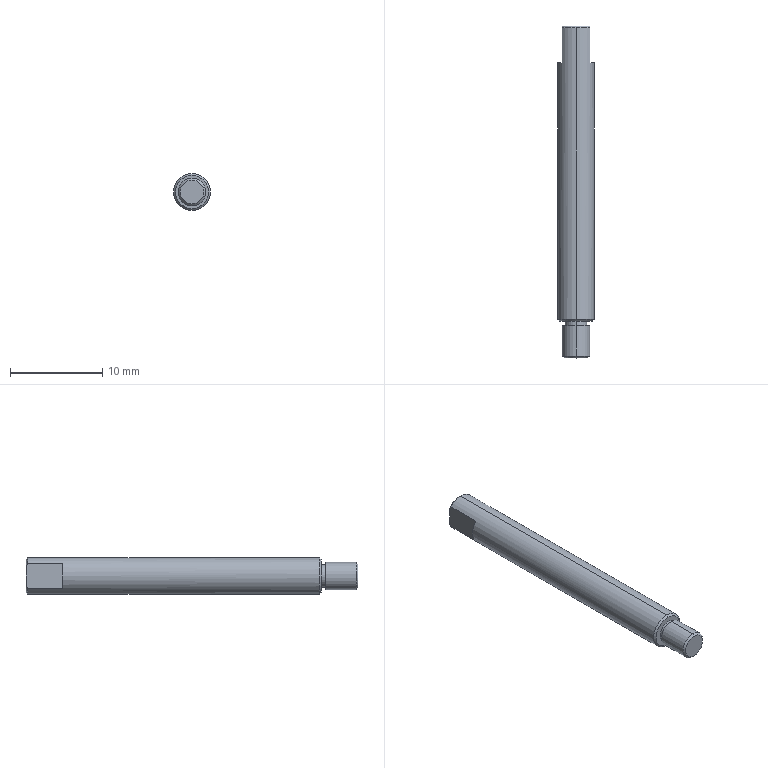Part | STEP file | 10000054026swp000-1 | 1 solid | 21 faces | box 4 x 36 x 4 mm | volume 421.312 mm3 | plane 8 | cone 7 | cylinder 6 | commonest cylinder face diameters 2.4 x2 3 x2 4 x2
STEP:
#1=CARTESIAN_POINT('',(0.,0.,-1.3));
#2=VERTEX_POINT('',#1);
#3=CARTESIAN_POINT('',(0.,0.,1.3));
#4=VERTEX_POINT('',#3);
#5=CARTESIAN_POINT('',(0.,0.,0.));
#6=DIRECTION('',(0.,-1.,0.));
#7=DIRECTION('',(0.,0.,1.));
#8=AXIS2_PLACEMENT_3D('',#5,#6,#7);
#9=CIRCLE('',#8,1.3);
#10=EDGE_CURVE('',#2,#4,#9,.T.);
#11=ORIENTED_EDGE('',*,*,#10,.F.);
#12=CARTESIAN_POINT('',(0.,0.2,-1.5));
#13=VERTEX_POINT('',#12);
#14=CARTESIAN_POINT('',(0.,0.2,-1.5));
#15=DIRECTION('',(0.,0.7071,-0.7071));
#16=VECTOR('',#15,1000.);
#17=LINE('',#14,#16);
#18=EDGE_CURVE('',#2,#13,#17,.T.);
#19=ORIENTED_EDGE('',*,*,#18,.T.);
#20=CARTESIAN_POINT('',(0.,0.2,1.5));
#21=VERTEX_POINT('',#20);
#22=CARTESIAN_POINT('',(0.,0.2,0.));
#23=DIRECTION('',(0.,1.,0.));
#24=DIRECTION('',(0.,0.,1.));
#25=AXIS2_PLACEMENT_3D('',#22,#23,#24);
#26=CIRCLE('',#25,1.5);
#27=EDGE_CURVE('',#21,#13,#26,.T.);
#28=ORIENTED_EDGE('',*,*,#27,.F.);
#29=CARTESIAN_POINT('',(0.,0.2,1.5));
#30=DIRECTION('',(0.,0.7071,0.7071));
#31=VECTOR('',#30,1000.);
#32=LINE('',#29,#31);
#33=EDGE_CURVE('',#4,#21,#32,.T.);
#34=ORIENTED_EDGE('',*,*,#33,.F.);
#35=EDGE_LOOP('',(#11,#19,#28,#34));
#36=FACE_OUTER_BOUND('',#35,.T.);
#37=CARTESIAN_POINT('',(0.,0.2,0.));
#38=DIRECTION('',(0.,1.,0.));
#39=DIRECTION('',(0.,0.,1.));
#40=AXIS2_PLACEMENT_3D('',#37,#38,#39);
#41=CONICAL_SURFACE('',#40,1.5,0.7854);
#42=ADVANCED_FACE('',(#36),#41,.T.);
#43=CARTESIAN_POINT('',(0.,4.,-1.8));
#44=VERTEX_POINT('',#43);
#45=CARTESIAN_POINT('',(0.,4.,1.8));
#46=VERTEX_POINT('',#45);
#47=CARTESIAN_POINT('',(0.,4.,0.));
#48=DIRECTION('',(0.,-1.,0.));
#49=DIRECTION('',(0.,0.,1.));
#50=AXIS2_PLACEMENT_3D('',#47,#48,#49);
#51=CIRCLE('',#50,1.8);
#52=EDGE_CURVE('',#44,#46,#51,.T.);
#53=ORIENTED_EDGE('',*,*,#52,.F.);
#54=CARTESIAN_POINT('',(0.,4.2,-2.));
#55=VERTEX_POINT('',#54);
#56=CARTESIAN_POINT('',(0.,4.2,-2.));
#57=DIRECTION('',(0.,0.7071,-0.7071));
#58=VECTOR('',#57,1000.);
#59=LINE('',#56,#58);
#60=EDGE_CURVE('',#44,#55,#59,.T.);
#61=ORIENTED_EDGE('',*,*,#60,.T.);
#62=CARTESIAN_POINT('',(0.,4.2,2.));
#63=VERTEX_POINT('',#62);
#64=CARTESIAN_POINT('',(0.,4.2,0.));
#65=DIRECTION('',(0.,1.,0.));
#66=DIRECTION('',(0.,0.,1.));
#67=AXIS2_PLACEMENT_3D('',#64,#65,#66);
#68=CIRCLE('',#67,2.);
#69=EDGE_CURVE('',#63,#55,#68,.T.);
#70=ORIENTED_EDGE('',*,*,#69,.F.);
#71=CARTESIAN_POINT('',(0.,4.2,2.));
#72=DIRECTION('',(0.,0.7071,0.7071));
#73=VECTOR('',#72,1000.);
#74=LINE('',#71,#73);
#75=EDGE_CURVE('',#46,#63,#74,.T.);
#76=ORIENTED_EDGE('',*,*,#75,.F.);
#77=EDGE_LOOP('',(#53,#61,#70,#76));
#78=FACE_OUTER_BOUND('',#77,.T.);
#79=CARTESIAN_POINT('',(0.,4.2,0.));
#80=DIRECTION('',(0.,1.,0.));
#81=DIRECTION('',(0.,0.,1.));
#82=AXIS2_PLACEMENT_3D('',#79,#80,#81);
#83=CONICAL_SURFACE('',#82,2.,0.7854);
#84=ADVANCED_FACE('',(#78),#83,.T.);
#85=CARTESIAN_POINT('',(0.,36.,-1.8));
#86=VERTEX_POINT('',#85);
#87=CARTESIAN_POINT('',(-1.5,36.,-0.995));
#88=VERTEX_POINT('',#87);
#89=CARTESIAN_POINT('',(0.,36.,0.));
#90=DIRECTION('',(0.,1.,0.));
#91=DIRECTION('',(0.,0.,-1.));
#92=AXIS2_PLACEMENT_3D('',#89,#90,#91);
#93=CIRCLE('',#92,1.8);
#94=EDGE_CURVE('',#86,#88,#93,.T.);
#95=ORIENTED_EDGE('',*,*,#94,.F.);
#96=CARTESIAN_POINT('',(0.,35.8,-2.));
#97=VERTEX_POINT('',#96);
#98=CARTESIAN_POINT('',(0.,36.,-1.8));
#99=DIRECTION('',(0.,-0.7071,-0.7071));
#100=VECTOR('',#99,1000.);
#101=LINE('',#98,#100);
#102=EDGE_CURVE('',#86,#97,#101,.T.);
#103=ORIENTED_EDGE('',*,*,#102,.T.);
#104=CARTESIAN_POINT('',(-1.5,35.8,-1.323));
#105=VERTEX_POINT('',#104);
#106=CARTESIAN_POINT('',(0.,35.8,0.));
#107=DIRECTION('',(0.,-1.,0.));
#108=DIRECTION('',(0.,0.,-1.));
#109=AXIS2_PLACEMENT_3D('',#106,#107,#108);
#110=CIRCLE('',#109,2.);
#111=EDGE_CURVE('',#105,#97,#110,.T.);
#112=ORIENTED_EDGE('',*,*,#111,.F.);
#113=CARTESIAN_POINT('',(-1.5,36.,-0.995));
#114=CARTESIAN_POINT('',(-1.5,35.938,-1.107));
#115=CARTESIAN_POINT('',(-1.5,35.871,-1.216));
#116=CARTESIAN_POINT('',(-1.5,35.8,-1.323));
#117=B_SPLINE_CURVE_WITH_KNOTS('',3,(#113,#114,#115,#116),.UNSPECIFIED.,.F.,.F.,(4,4),(0.,0.0003841),.UNSPECIFIED.);
#118=EDGE_CURVE('',#88,#105,#117,.T.);
#119=ORIENTED_EDGE('',*,*,#118,.F.);
#120=EDGE_LOOP('',(#95,#103,#112,#119));
#121=FACE_OUTER_BOUND('',#120,.T.);
#122=CARTESIAN_POINT('',(0.,36.,0.));
#123=DIRECTION('',(0.,-1.,0.));
#124=DIRECTION('',(0.,0.,-1.));
#125=AXIS2_PLACEMENT_3D('',#122,#123,#124);
#126=CONICAL_SURFACE('',#125,1.8,0.7854);
#127=ADVANCED_FACE('',(#121),#126,.T.);
#128=ORIENTED_EDGE('',*,*,#27,.T.);
#129=CARTESIAN_POINT('',(0.,3.5,-1.5));
#130=VERTEX_POINT('',#129);
#131=CARTESIAN_POINT('',(0.,0.,-1.5));
#132=DIRECTION('',(0.,1.,0.));
#133=VECTOR('',#132,1000.);
#134=LINE('',#131,#133);
#135=EDGE_CURVE('',#13,#130,#134,.T.);
#136=ORIENTED_EDGE('',*,*,#135,.T.);
#137=CARTESIAN_POINT('',(0.,3.5,1.5));
#138=VERTEX_POINT('',#137);
#139=CARTESIAN_POINT('',(0.,3.5,0.));
#140=DIRECTION('',(0.,1.,0.));
#141=DIRECTION('',(0.,0.,1.));
#142=AXIS2_PLACEMENT_3D('',#139,#140,#141);
#143=CIRCLE('',#142,1.5);
#144=EDGE_CURVE('',#138,#130,#143,.T.);
#145=ORIENTED_EDGE('',*,*,#144,.F.);
#146=CARTESIAN_POINT('',(0.,0.,1.5));
#147=DIRECTION('',(0.,1.,0.));
#148=VECTOR('',#147,1000.);
#149=LINE('',#146,#148);
#150=EDGE_CURVE('',#21,#138,#149,.T.);
#151=ORIENTED_EDGE('',*,*,#150,.F.);
#152=EDGE_LOOP('',(#128,#136,#145,#151));
#153=FACE_OUTER_BOUND('',#152,.T.);
#154=CARTESIAN_POINT('',(0.,0.,0.));
#155=DIRECTION('',(0.,1.,0.));
#156=DIRECTION('',(0.,0.,1.));
#157=AXIS2_PLACEMENT_3D('',#154,#155,#156);
#158=CYLINDRICAL_SURFACE('',#157,1.5);
#159=ADVANCED_FACE('',(#153),#158,.T.);
#160=CARTESIAN_POINT('',(0.,3.5,1.2));
#161=VERTEX_POINT('',#160);
#162=CARTESIAN_POINT('',(0.,3.5,-1.2));
#163=VERTEX_POINT('',#162);
#164=CARTESIAN_POINT('',(0.,3.5,0.));
#165=DIRECTION('',(0.,1.,0.));
#166=DIRECTION('',(0.,0.,1.));
#167=AXIS2_PLACEMENT_3D('',#164,#165,#166);
#168=CIRCLE('',#167,1.2);
#169=EDGE_CURVE('',#161,#163,#168,.T.);
#170=ORIENTED_EDGE('',*,*,#169,.T.);
#171=CARTESIAN_POINT('',(0.,4.,-1.2));
#172=VERTEX_POINT('',#171);
#173=CARTESIAN_POINT('',(0.,0.,-1.2));
#174=DIRECTION('',(0.,1.,0.));
#175=VECTOR('',#174,1000.);
#176=LINE('',#173,#175);
#177=EDGE_CURVE('',#163,#172,#176,.T.);
#178=ORIENTED_EDGE('',*,*,#177,.T.);
#179=CARTESIAN_POINT('',(0.,4.,1.2));
#180=VERTEX_POINT('',#179);
#181=CARTESIAN_POINT('',(0.,4.,0.));
#182=DIRECTION('',(0.,1.,0.));
#183=DIRECTION('',(0.,0.,1.));
#184=AXIS2_PLACEMENT_3D('',#181,#182,#183);
#185=CIRCLE('',#184,1.2);
#186=EDGE_CURVE('',#180,#172,#185,.T.);
#187=ORIENTED_EDGE('',*,*,#186,.F.);
#188=CARTESIAN_POINT('',(0.,0.,1.2));
#189=DIRECTION('',(0.,1.,0.));
#190=VECTOR('',#189,1000.);
#191=LINE('',#188,#190);
#192=EDGE_CURVE('',#161,#180,#191,.T.);
#193=ORIENTED_EDGE('',*,*,#192,.F.);
#194=EDGE_LOOP('',(#170,#178,#187,#193));
#195=FACE_OUTER_BOUND('',#194,.T.);
#196=CARTESIAN_POINT('',(0.,0.,0.));
#197=DIRECTION('',(0.,1.,0.));
#198=DIRECTION('',(0.,0.,1.));
#199=AXIS2_PLACEMENT_3D('',#196,#197,#198);
#200=CYLINDRICAL_SURFACE('',#199,1.2);
#201=ADVANCED_FACE('',(#195),#200,.T.);
#202=ORIENTED_EDGE('',*,*,#69,.T.);
#203=CARTESIAN_POINT('',(0.,0.,-2.));
#204=DIRECTION('',(0.,1.,0.));
#205=VECTOR('',#204,1000.);
#206=LINE('',#203,#205);
#207=EDGE_CURVE('',#55,#97,#206,.T.);
#208=ORIENTED_EDGE('',*,*,#207,.T.);
#209=CARTESIAN_POINT('',(1.5,35.8,-1.323));
#210=VERTEX_POINT('',#209);
#211=CARTESIAN_POINT('',(0.,35.8,0.));
#212=DIRECTION('',(0.,-1.,0.));
#213=DIRECTION('',(0.,0.,-1.));
#214=AXIS2_PLACEMENT_3D('',#211,#212,#213);
#215=CIRCLE('',#214,2.);
#216=EDGE_CURVE('',#97,#210,#215,.T.);
#217=ORIENTED_EDGE('',*,*,#216,.T.);
#218=CARTESIAN_POINT('',(1.5,32.,-1.323));
#219=VERTEX_POINT('',#218);
#220=CARTESIAN_POINT('',(1.5,32.,-1.323));
#221=DIRECTION('',(0.,1.,0.));
#222=VECTOR('',#221,1000.);
#223=LINE('',#220,#222);
#224=EDGE_CURVE('',#219,#210,#223,.T.);
#225=ORIENTED_EDGE('',*,*,#224,.F.);
#226=CARTESIAN_POINT('',(1.5,32.,1.323));
#227=VERTEX_POINT('',#226);
#228=CARTESIAN_POINT('',(0.,32.,0.));
#229=DIRECTION('',(0.,1.,0.));
#230=DIRECTION('',(0.,0.,1.));
#231=AXIS2_PLACEMENT_3D('',#228,#229,#230);
#232=CIRCLE('',#231,2.);
#233=EDGE_CURVE('',#227,#219,#232,.T.);
#234=ORIENTED_EDGE('',*,*,#233,.F.);
#235=CARTESIAN_POINT('',(1.5,35.8,1.323));
#236=VERTEX_POINT('',#235);
#237=CARTESIAN_POINT('',(1.5,32.,1.323));
#238=DIRECTION('',(0.,1.,0.));
#239=VECTOR('',#238,1000.);
#240=LINE('',#237,#239);
#241=EDGE_CURVE('',#227,#236,#240,.T.);
#242=ORIENTED_EDGE('',*,*,#241,.T.);
#243=CARTESIAN_POINT('',(0.,35.8,2.));
#244=VERTEX_POINT('',#243);
#245=CARTESIAN_POINT('',(0.,35.8,0.));
#246=DIRECTION('',(0.,-1.,0.));
#247=DIRECTION('',(0.,0.,-1.));
#248=AXIS2_PLACEMENT_3D('',#245,#246,#247);
#249=CIRCLE('',#248,2.);
#250=EDGE_CURVE('',#236,#244,#249,.T.);
#251=ORIENTED_EDGE('',*,*,#250,.T.);
#252=CARTESIAN_POINT('',(0.,0.,2.));
#253=DIRECTION('',(0.,1.,0.));
#254=VECTOR('',#253,1000.);
#255=LINE('',#252,#254);
#256=EDGE_CURVE('',#63,#244,#255,.T.);
#257=ORIENTED_EDGE('',*,*,#256,.F.);
#258=EDGE_LOOP('',(#202,#208,#217,#225,#234,#242,#251,#257));
#259=FACE_OUTER_BOUND('',#258,.T.);
#260=CARTESIAN_POINT('',(0.,0.,0.));
#261=DIRECTION('',(0.,1.,0.));
#262=DIRECTION('',(0.,0.,1.));
#263=AXIS2_PLACEMENT_3D('',#260,#261,#262);
#264=CYLINDRICAL_SURFACE('',#263,2.);
#265=ADVANCED_FACE('',(#259),#264,.T.);
#266=CARTESIAN_POINT('',(0.,4.,0.));
#267=DIRECTION('',(0.,-1.,0.));
#268=DIRECTION('',(0.,0.,1.));
#269=AXIS2_PLACEMENT_3D('',#266,#267,#268);
#270=CIRCLE('',#269,1.8);
#271=EDGE_CURVE('',#46,#44,#270,.T.);
#272=ORIENTED_EDGE('',*,*,#271,.T.);
#273=ORIENTED_EDGE('',*,*,#52,.T.);
#274=EDGE_LOOP('',(#272,#273));
#275=FACE_OUTER_BOUND('',#274,.T.);
#276=ORIENTED_EDGE('',*,*,#186,.T.);
#277=CARTESIAN_POINT('',(0.,4.,0.));
#278=DIRECTION('',(0.,1.,0.));
#279=DIRECTION('',(0.,0.,1.));
#280=AXIS2_PLACEMENT_3D('',#277,#278,#279);
#281=CIRCLE('',#280,1.2);
#282=EDGE_CURVE('',#172,#180,#281,.T.);
#283=ORIENTED_EDGE('',*,*,#282,.T.);
#284=EDGE_LOOP('',(#276,#283));
#285=FACE_BOUND('',#284,.T.);
#286=CARTESIAN_POINT('',(1.5,4.,0.));
#287=DIRECTION('',(0.,1.,0.));
#288=DIRECTION('',(0.,0.,1.));
#289=AXIS2_PLACEMENT_3D('',#286,#287,#288);
#290=PLANE('',#289);
#291=ADVANCED_FACE('',(#275,#285),#290,.F.);
#292=ORIENTED_EDGE('',*,*,#207,.F.);
#293=CARTESIAN_POINT('',(0.,4.2,0.));
#294=DIRECTION('',(0.,1.,0.));
#295=DIRECTION('',(0.,0.,1.));
#296=AXIS2_PLACEMENT_3D('',#293,#294,#295);
#297=CIRCLE('',#296,2.);
#298=EDGE_CURVE('',#55,#63,#297,.T.);
#299=ORIENTED_EDGE('',*,*,#298,.T.);
#300=ORIENTED_EDGE('',*,*,#256,.T.);
#301=CARTESIAN_POINT('',(-1.5,35.8,1.323));
#302=VERTEX_POINT('',#301);
#303=CARTESIAN_POINT('',(0.,35.8,0.));
#304=DIRECTION('',(0.,-1.,0.));
#305=DIRECTION('',(0.,0.,-1.));
#306=AXIS2_PLACEMENT_3D('',#303,#304,#305);
#307=CIRCLE('',#306,2.);
#308=EDGE_CURVE('',#244,#302,#307,.T.);
#309=ORIENTED_EDGE('',*,*,#308,.T.);
#310=CARTESIAN_POINT('',(-1.5,32.,1.323));
#311=VERTEX_POINT('',#310);
#312=CARTESIAN_POINT('',(-1.5,32.,1.323));
#313=DIRECTION('',(0.,1.,0.));
#314=VECTOR('',#313,1000.);
#315=LINE('',#312,#314);
#316=EDGE_CURVE('',#311,#302,#315,.T.);
#317=ORIENTED_EDGE('',*,*,#316,.F.);
#318=CARTESIAN_POINT('',(-1.5,32.,-1.323));
#319=VERTEX_POINT('',#318);
#320=CARTESIAN_POINT('',(0.,32.,0.));
#321=DIRECTION('',(0.,1.,0.));
#322=DIRECTION('',(0.,0.,1.));
#323=AXIS2_PLACEMENT_3D('',#320,#321,#322);
#324=CIRCLE('',#323,2.);
#325=EDGE_CURVE('',#319,#311,#324,.T.);
#326=ORIENTED_EDGE('',*,*,#325,.F.);
#327=CARTESIAN_POINT('',(-1.5,32.,-1.323));
#328=DIRECTION('',(0.,1.,0.));
#329=VECTOR('',#328,1000.);
#330=LINE('',#327,#329);
#331=EDGE_CURVE('',#319,#105,#330,.T.);
#332=ORIENTED_EDGE('',*,*,#331,.T.);
#333=ORIENTED_EDGE('',*,*,#111,.T.);
#334=EDGE_LOOP('',(#292,#299,#300,#309,#317,#326,#332,#333));
#335=FACE_OUTER_BOUND('',#334,.T.);
#336=CARTESIAN_POINT('',(0.,0.,0.));
#337=DIRECTION('',(0.,1.,0.));
#338=DIRECTION('',(0.,0.,1.));
#339=AXIS2_PLACEMENT_3D('',#336,#337,#338);
#340=CYLINDRICAL_SURFACE('',#339,2.);
#341=ADVANCED_FACE('',(#335),#340,.T.);
#342=CARTESIAN_POINT('',(1.5,36.,-0.995));
#343=VERTEX_POINT('',#342);
#344=CARTESIAN_POINT('',(1.5,36.,0.995));
#345=VERTEX_POINT('',#344);
#346=CARTESIAN_POINT('',(1.5,36.,-1.323));
#347=DIRECTION('',(0.,0.,1.));
#348=VECTOR('',#347,1000.);
#349=LINE('',#346,#348);
#350=EDGE_CURVE('',#343,#345,#349,.T.);
#351=ORIENTED_EDGE('',*,*,#350,.F.);
#352=CARTESIAN_POINT('',(0.,36.,0.));
#353=DIRECTION('',(0.,1.,0.));
#354=DIRECTION('',(0.,0.,-1.));
#355=AXIS2_PLACEMENT_3D('',#352,#353,#354);
#356=CIRCLE('',#355,1.8);
#357=EDGE_CURVE('',#343,#86,#356,.T.);
#358=ORIENTED_EDGE('',*,*,#357,.T.);
#359=ORIENTED_EDGE('',*,*,#94,.T.);
#360=CARTESIAN_POINT('',(-1.5,36.,0.995));
#361=VERTEX_POINT('',#360);
#362=CARTESIAN_POINT('',(-1.5,36.,-1.323));
#363=DIRECTION('',(0.,0.,-1.));
#364=VECTOR('',#363,1000.);
#365=LINE('',#362,#364);
#366=EDGE_CURVE('',#361,#88,#365,.T.);
#367=ORIENTED_EDGE('',*,*,#366,.F.);
#368=CARTESIAN_POINT('',(0.,36.,0.));
#369=DIRECTION('',(0.,1.,0.));
#370=DIRECTION('',(0.,0.,-1.));
#371=AXIS2_PLACEMENT_3D('',#368,#369,#370);
#372=CIRCLE('',#371,1.8);
#373=EDGE_CURVE('',#361,#345,#372,.T.);
#374=ORIENTED_EDGE('',*,*,#373,.T.);
#375=EDGE_LOOP('',(#351,#358,#359,#367,#374));
#376=FACE_OUTER_BOUND('',#375,.T.);
#377=CARTESIAN_POINT('',(2.,36.,0.));
#378=DIRECTION('',(0.,-1.,0.));
#379=DIRECTION('',(0.,0.,-1.));
#380=AXIS2_PLACEMENT_3D('',#377,#378,#379);
#381=PLANE('',#380);
#382=ADVANCED_FACE('',(#376),#381,.F.);
#383=ORIENTED_EDGE('',*,*,#366,.T.);
#384=ORIENTED_EDGE('',*,*,#118,.T.);
#385=ORIENTED_EDGE('',*,*,#331,.F.);
#386=CARTESIAN_POINT('',(-1.5,32.,-1.323));
#387=DIRECTION('',(0.,0.,-1.));
#388=VECTOR('',#387,1000.);
#389=LINE('',#386,#388);
#390=EDGE_CURVE('',#311,#319,#389,.T.);
#391=ORIENTED_EDGE('',*,*,#390,.F.);
#392=ORIENTED_EDGE('',*,*,#316,.T.);
#393=CARTESIAN_POINT('',(-1.5,35.8,1.323));
#394=CARTESIAN_POINT('',(-1.5,35.871,1.216));
#395=CARTESIAN_POINT('',(-1.5,35.938,1.107));
#396=CARTESIAN_POINT('',(-1.5,36.,0.995));
#397=B_SPLINE_CURVE_WITH_KNOTS('',3,(#393,#394,#395,#396),.UNSPECIFIED.,.F.,.F.,(4,4),(0.,0.0003841),.UNSPECIFIED.);
#398=EDGE_CURVE('',#302,#361,#397,.T.);
#399=ORIENTED_EDGE('',*,*,#398,.T.);
#400=EDGE_LOOP('',(#383,#384,#385,#391,#392,#399));
#401=FACE_OUTER_BOUND('',#400,.T.);
#402=CARTESIAN_POINT('',(-1.5,32.,-1.323));
#403=DIRECTION('',(1.,0.,0.));
#404=DIRECTION('',(0.,0.,-1.));
#405=AXIS2_PLACEMENT_3D('',#402,#403,#404);
#406=PLANE('',#405);
#407=ADVANCED_FACE('',(#401),#406,.F.);
#408=ORIENTED_EDGE('',*,*,#325,.T.);
#409=ORIENTED_EDGE('',*,*,#390,.T.);
#410=EDGE_LOOP('',(#408,#409));
#411=FACE_OUTER_BOUND('',#410,.T.);
#412=CARTESIAN_POINT('',(0.,32.,0.));
#413=DIRECTION('',(0.,1.,0.));
#414=DIRECTION('',(0.,0.,1.));
#415=AXIS2_PLACEMENT_3D('',#412,#413,#414);
#416=PLANE('',#415);
#417=ADVANCED_FACE('',(#411),#416,.T.);
#418=ORIENTED_EDGE('',*,*,#224,.T.);
#419=CARTESIAN_POINT('',(1.5,35.8,-1.323));
#420=CARTESIAN_POINT('',(1.5,35.871,-1.216));
#421=CARTESIAN_POINT('',(1.5,35.938,-1.107));
#422=CARTESIAN_POINT('',(1.5,36.,-0.995));
#423=B_SPLINE_CURVE_WITH_KNOTS('',3,(#419,#420,#421,#422),.UNSPECIFIED.,.F.,.F.,(4,4),(0.,0.0003841),.UNSPECIFIED.);
#424=EDGE_CURVE('',#210,#343,#423,.T.);
#425=ORIENTED_EDGE('',*,*,#424,.T.);
#426=ORIENTED_EDGE('',*,*,#350,.T.);
#427=CARTESIAN_POINT('',(1.5,36.,0.995));
#428=CARTESIAN_POINT('',(1.5,35.938,1.107));
#429=CARTESIAN_POINT('',(1.5,35.871,1.216));
#430=CARTESIAN_POINT('',(1.5,35.8,1.323));
#431=B_SPLINE_CURVE_WITH_KNOTS('',3,(#427,#428,#429,#430),.UNSPECIFIED.,.F.,.F.,(4,4),(0.,0.0003841),.UNSPECIFIED.);
#432=EDGE_CURVE('',#345,#236,#431,.T.);
#433=ORIENTED_EDGE('',*,*,#432,.T.);
#434=ORIENTED_EDGE('',*,*,#241,.F.);
#435=CARTESIAN_POINT('',(1.5,32.,-1.323));
#436=DIRECTION('',(0.,0.,1.));
#437=VECTOR('',#436,1000.);
#438=LINE('',#435,#437);
#439=EDGE_CURVE('',#219,#227,#438,.T.);
#440=ORIENTED_EDGE('',*,*,#439,.F.);
#441=EDGE_LOOP('',(#418,#425,#426,#433,#434,#440));
#442=FACE_OUTER_BOUND('',#441,.T.);
#443=CARTESIAN_POINT('',(1.5,32.,-1.323));
#444=DIRECTION('',(-1.,0.,0.));
#445=DIRECTION('',(0.,0.,1.));
#446=AXIS2_PLACEMENT_3D('',#443,#444,#445);
#447=PLANE('',#446);
#448=ADVANCED_FACE('',(#442),#447,.F.);
#449=ORIENTED_EDGE('',*,*,#233,.T.);
#450=ORIENTED_EDGE('',*,*,#439,.T.);
#451=EDGE_LOOP('',(#449,#450));
#452=FACE_OUTER_BOUND('',#451,.T.);
#453=CARTESIAN_POINT('',(0.,32.,0.));
#454=DIRECTION('',(0.,1.,0.));
#455=DIRECTION('',(0.,0.,1.));
#456=AXIS2_PLACEMENT_3D('',#453,#454,#455);
#457=PLANE('',#456);
#458=ADVANCED_FACE('',(#452),#457,.T.);
#459=ORIENTED_EDGE('',*,*,#177,.F.);
#460=CARTESIAN_POINT('',(0.,3.5,0.));
#461=DIRECTION('',(0.,1.,0.));
#462=DIRECTION('',(0.,0.,1.));
#463=AXIS2_PLACEMENT_3D('',#460,#461,#462);
#464=CIRCLE('',#463,1.2);
#465=EDGE_CURVE('',#163,#161,#464,.T.);
#466=ORIENTED_EDGE('',*,*,#465,.T.);
#467=ORIENTED_EDGE('',*,*,#192,.T.);
#468=ORIENTED_EDGE('',*,*,#282,.F.);
#469=EDGE_LOOP('',(#459,#466,#467,#468));
#470=FACE_OUTER_BOUND('',#469,.T.);
#471=CARTESIAN_POINT('',(0.,0.,0.));
#472=DIRECTION('',(0.,1.,0.));
#473=DIRECTION('',(0.,0.,1.));
#474=AXIS2_PLACEMENT_3D('',#471,#472,#473);
#475=CYLINDRICAL_SURFACE('',#474,1.2);
#476=ADVANCED_FACE('',(#470),#475,.T.);
#477=ORIENTED_EDGE('',*,*,#144,.T.);
#478=CARTESIAN_POINT('',(0.,3.5,0.));
#479=DIRECTION('',(0.,1.,0.));
#480=DIRECTION('',(0.,0.,1.));
#481=AXIS2_PLACEMENT_3D('',#478,#479,#480);
#482=CIRCLE('',#481,1.5);
#483=EDGE_CURVE('',#130,#138,#482,.T.);
#484=ORIENTED_EDGE('',*,*,#483,.T.);
#485=EDGE_LOOP('',(#477,#484));
#486=FACE_OUTER_BOUND('',#485,.T.);
#487=ORIENTED_EDGE('',*,*,#169,.F.);
#488=ORIENTED_EDGE('',*,*,#465,.F.);
#489=EDGE_LOOP('',(#487,#488));
#490=FACE_BOUND('',#489,.T.);
#491=CARTESIAN_POINT('',(1.5,3.5,0.));
#492=DIRECTION('',(0.,1.,0.));
#493=DIRECTION('',(0.,0.,1.));
#494=AXIS2_PLACEMENT_3D('',#491,#492,#493);
#495=PLANE('',#494);
#496=ADVANCED_FACE('',(#486,#490),#495,.T.);
#497=CARTESIAN_POINT('',(0.,0.,0.));
#498=DIRECTION('',(0.,-1.,0.));
#499=DIRECTION('',(0.,0.,1.));
#500=AXIS2_PLACEMENT_3D('',#497,#498,#499);
#501=CIRCLE('',#500,1.3);
#502=EDGE_CURVE('',#4,#2,#501,.T.);
#503=ORIENTED_EDGE('',*,*,#502,.T.);
#504=ORIENTED_EDGE('',*,*,#10,.T.);
#505=EDGE_LOOP('',(#503,#504));
#506=FACE_OUTER_BOUND('',#505,.T.);
#507=CARTESIAN_POINT('',(0.,0.,0.));
#508=DIRECTION('',(0.,1.,0.));
#509=DIRECTION('',(0.,0.,1.));
#510=AXIS2_PLACEMENT_3D('',#507,#508,#509);
#511=PLANE('',#510);
#512=ADVANCED_FACE('',(#506),#511,.F.);
#513=ORIENTED_EDGE('',*,*,#135,.F.);
#514=CARTESIAN_POINT('',(0.,0.2,0.));
#515=DIRECTION('',(0.,1.,0.));
#516=DIRECTION('',(0.,0.,1.));
#517=AXIS2_PLACEMENT_3D('',#514,#515,#516);
#518=CIRCLE('',#517,1.5);
#519=EDGE_CURVE('',#13,#21,#518,.T.);
#520=ORIENTED_EDGE('',*,*,#519,.T.);
#521=ORIENTED_EDGE('',*,*,#150,.T.);
#522=ORIENTED_EDGE('',*,*,#483,.F.);
#523=EDGE_LOOP('',(#513,#520,#521,#522));
#524=FACE_OUTER_BOUND('',#523,.T.);
#525=CARTESIAN_POINT('',(0.,0.,0.));
#526=DIRECTION('',(0.,1.,0.));
#527=DIRECTION('',(0.,0.,1.));
#528=AXIS2_PLACEMENT_3D('',#525,#526,#527);
#529=CYLINDRICAL_SURFACE('',#528,1.5);
#530=ADVANCED_FACE('',(#524),#529,.T.);
#531=ORIENTED_EDGE('',*,*,#102,.F.);
#532=ORIENTED_EDGE('',*,*,#357,.F.);
#533=ORIENTED_EDGE('',*,*,#424,.F.);
#534=ORIENTED_EDGE('',*,*,#216,.F.);
#535=EDGE_LOOP('',(#531,#532,#533,#534));
#536=FACE_OUTER_BOUND('',#535,.T.);
#537=CARTESIAN_POINT('',(0.,36.,0.));
#538=DIRECTION('',(0.,-1.,0.));
#539=DIRECTION('',(0.,0.,-1.));
#540=AXIS2_PLACEMENT_3D('',#537,#538,#539);
#541=CONICAL_SURFACE('',#540,1.8,0.7854);
#542=ADVANCED_FACE('',(#536),#541,.T.);
#543=ORIENTED_EDGE('',*,*,#398,.F.);
#544=ORIENTED_EDGE('',*,*,#308,.F.);
#545=ORIENTED_EDGE('',*,*,#250,.F.);
#546=ORIENTED_EDGE('',*,*,#432,.F.);
#547=ORIENTED_EDGE('',*,*,#373,.F.);
#548=EDGE_LOOP('',(#543,#544,#545,#546,#547));
#549=FACE_OUTER_BOUND('',#548,.T.);
#550=CARTESIAN_POINT('',(0.,36.,0.));
#551=DIRECTION('',(0.,-1.,0.));
#552=DIRECTION('',(0.,0.,-1.));
#553=AXIS2_PLACEMENT_3D('',#550,#551,#552);
#554=CONICAL_SURFACE('',#553,1.8,0.7854);
#555=ADVANCED_FACE('',(#549),#554,.T.);
#556=ORIENTED_EDGE('',*,*,#60,.F.);
#557=ORIENTED_EDGE('',*,*,#271,.F.);
#558=ORIENTED_EDGE('',*,*,#75,.T.);
#559=ORIENTED_EDGE('',*,*,#298,.F.);
#560=EDGE_LOOP('',(#556,#557,#558,#559));
#561=FACE_OUTER_BOUND('',#560,.T.);
#562=CARTESIAN_POINT('',(0.,4.2,0.));
#563=DIRECTION('',(0.,1.,0.));
#564=DIRECTION('',(0.,0.,1.));
#565=AXIS2_PLACEMENT_3D('',#562,#563,#564);
#566=CONICAL_SURFACE('',#565,2.,0.7854);
#567=ADVANCED_FACE('',(#561),#566,.T.);
#568=ORIENTED_EDGE('',*,*,#18,.F.);
#569=ORIENTED_EDGE('',*,*,#502,.F.);
#570=ORIENTED_EDGE('',*,*,#33,.T.);
#571=ORIENTED_EDGE('',*,*,#519,.F.);
#572=EDGE_LOOP('',(#568,#569,#570,#571));
#573=FACE_OUTER_BOUND('',#572,.T.);
#574=CARTESIAN_POINT('',(0.,0.2,0.));
#575=DIRECTION('',(0.,1.,0.));
#576=DIRECTION('',(0.,0.,1.));
#577=AXIS2_PLACEMENT_3D('',#574,#575,#576);
#578=CONICAL_SURFACE('',#577,1.5,0.7854);
#579=ADVANCED_FACE('',(#573),#578,.T.);
#580=CLOSED_SHELL('',(#42,#84,#127,#159,#201,#265,#291,#341,#382,#407,#417,#448,#458,#476,#496,#512,#530,#542,#555,#567,#579));
#581=MANIFOLD_SOLID_BREP('',#580);
#582=CARTESIAN_POINT('',(0.,0.,0.));
#583=DIRECTION('',(0.,0.,1.));
#584=DIRECTION('',(1.,0.,0.));
#585=AXIS2_PLACEMENT_3D('',#582,#583,#584);
#586=(LENGTH_UNIT()NAMED_UNIT(*)SI_UNIT(.MILLI.,.METRE.));
#587=UNCERTAINTY_MEASURE_WITH_UNIT(LENGTH_MEASURE(0.00001),#586,'','');
#588=(NAMED_UNIT(*)PLANE_ANGLE_UNIT()SI_UNIT($,.RADIAN.));
#589=(NAMED_UNIT(*)SI_UNIT($,.STERADIAN.)SOLID_ANGLE_UNIT());
#590=(GEOMETRIC_REPRESENTATION_CONTEXT(3)GLOBAL_UNCERTAINTY_ASSIGNED_CONTEXT((#587))GLOBAL_UNIT_ASSIGNED_CONTEXT((#586,#588,#589))REPRESENTATION_CONTEXT('',''));
#591=ADVANCED_BREP_SHAPE_REPRESENTATION('',(#581,#585),#590);